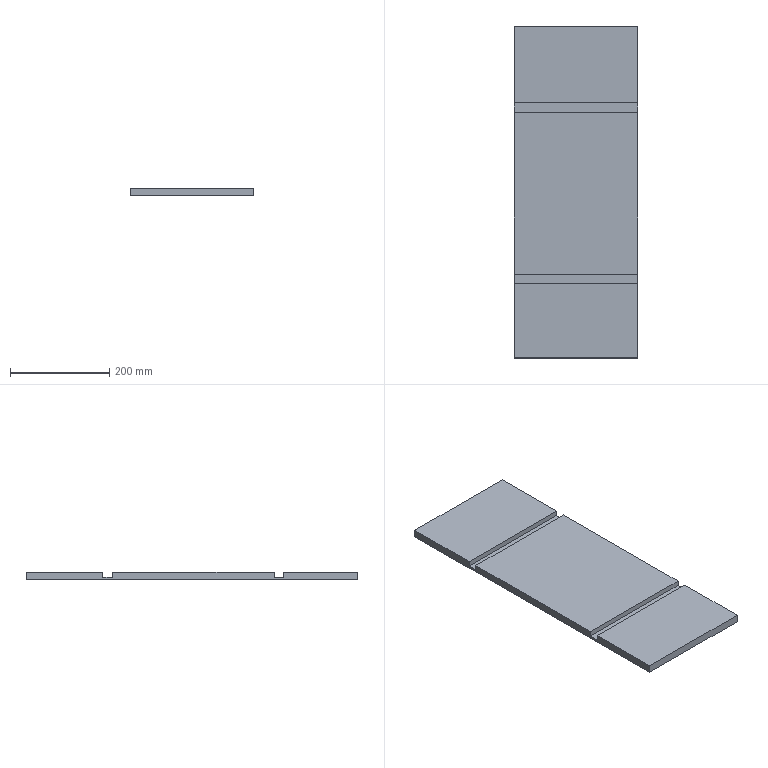Part | STEP file | Superstructure_3 | 1 solid | 14 faces | box 250 x 670 x 16 mm | volume 2577227 mm3 | plane 14
STEP:
#1=CARTESIAN_POINT('',(0.,0.,0.));
#2=DIRECTION('',(0.,0.,1.));
#3=DIRECTION('',(1.,0.,0.));
#4=AXIS2_PLACEMENT_3D('',#1,#2,#3);
#5=CARTESIAN_POINT('',(-125.,335.,0.));
#6=VERTEX_POINT('',#5);
#7=CARTESIAN_POINT('',(-125.,335.,-16.));
#8=VERTEX_POINT('',#7);
#9=CARTESIAN_POINT('',(-125.,335.,0.));
#10=DIRECTION('',(0.,0.,-1.));
#11=VECTOR('',#10,1.);
#12=LINE('',#9,#11);
#13=CARTESIAN_POINT('',(-125.,335.,0.));
#14=DIRECTION('',(1.,0.,0.));
#15=DIRECTION('',(0.,0.,-1.));
#16=AXIS2_PLACEMENT_3D('',#13,#14,#15);
#17=PLANE('',#16);
#18=CARTESIAN_POINT('',(0.,0.));
#19=DIRECTION('',(1.,0.));
#20=VECTOR('',#19,1.);
#21=LINE('',#18,#20);
#22=(GEOMETRIC_REPRESENTATION_CONTEXT(2)PARAMETRIC_REPRESENTATION_CONTEXT()REPRESENTATION_CONTEXT('',''));
#23=DEFINITIONAL_REPRESENTATION('',(#21),#22);
#24=PCURVE('',#17,#23);
#25=CARTESIAN_POINT('',(0.,335.,-8.));
#26=DIRECTION('',(0.,1.,0.));
#27=DIRECTION('',(0.,0.,1.));
#28=AXIS2_PLACEMENT_3D('',#25,#26,#27);
#29=PLANE('',#28);
#30=CARTESIAN_POINT('',(8.,-125.));
#31=DIRECTION('',(-1.,0.));
#32=VECTOR('',#31,1.);
#33=LINE('',#30,#32);
#34=(GEOMETRIC_REPRESENTATION_CONTEXT(2)PARAMETRIC_REPRESENTATION_CONTEXT()REPRESENTATION_CONTEXT('',''));
#35=DEFINITIONAL_REPRESENTATION('',(#33),#34);
#36=PCURVE('',#29,#35);
#37=SURFACE_CURVE('',#12,(#24,#36),.PCURVE_S1.);
#38=EDGE_CURVE('',#6,#8,#37,.T.);
#39=ORIENTED_EDGE('',*,*,#38,.F.);
#40=CARTESIAN_POINT('',(-125.,180.,0.));
#41=VERTEX_POINT('',#40);
#42=CARTESIAN_POINT('',(-125.,335.,0.));
#43=DIRECTION('',(0.,-1.,0.));
#44=VECTOR('',#43,1.);
#45=LINE('',#42,#44);
#46=CARTESIAN_POINT('',(0.,0.));
#47=DIRECTION('',(0.,-1.));
#48=VECTOR('',#47,1.);
#49=LINE('',#46,#48);
#50=(GEOMETRIC_REPRESENTATION_CONTEXT(2)PARAMETRIC_REPRESENTATION_CONTEXT()REPRESENTATION_CONTEXT('',''));
#51=DEFINITIONAL_REPRESENTATION('',(#49),#50);
#52=PCURVE('',#17,#51);
#53=CARTESIAN_POINT('',(125.,335.,0.));
#54=DIRECTION('',(0.,0.,-1.));
#55=DIRECTION('',(-1.,0.,0.));
#56=AXIS2_PLACEMENT_3D('',#53,#54,#55);
#57=PLANE('',#56);
#58=CARTESIAN_POINT('',(250.,0.));
#59=DIRECTION('',(0.,-1.));
#60=VECTOR('',#59,1.);
#61=LINE('',#58,#60);
#62=(GEOMETRIC_REPRESENTATION_CONTEXT(2)PARAMETRIC_REPRESENTATION_CONTEXT()REPRESENTATION_CONTEXT('',''));
#63=DEFINITIONAL_REPRESENTATION('',(#61),#62);
#64=PCURVE('',#57,#63);
#65=SURFACE_CURVE('',#45,(#52,#64),.PCURVE_S1.);
#66=EDGE_CURVE('',#6,#41,#65,.T.);
#67=ORIENTED_EDGE('',*,*,#66,.T.);
#68=CARTESIAN_POINT('',(-125.,180.,-10.65));
#69=VERTEX_POINT('',#68);
#70=CARTESIAN_POINT('',(-125.,180.,-2.663));
#71=DIRECTION('',(0.,0.,1.));
#72=VECTOR('',#71,1.);
#73=LINE('',#70,#72);
#74=CARTESIAN_POINT('',(2.663,-155.));
#75=DIRECTION('',(-1.,0.));
#76=VECTOR('',#75,1.);
#77=LINE('',#74,#76);
#78=(GEOMETRIC_REPRESENTATION_CONTEXT(2)PARAMETRIC_REPRESENTATION_CONTEXT()REPRESENTATION_CONTEXT('',''));
#79=DEFINITIONAL_REPRESENTATION('',(#77),#78);
#80=PCURVE('',#17,#79);
#81=CARTESIAN_POINT('',(0.,180.,-5.325));
#82=DIRECTION('',(0.,1.,0.));
#83=DIRECTION('',(0.,0.,1.));
#84=AXIS2_PLACEMENT_3D('',#81,#82,#83);
#85=PLANE('',#84);
#86=CARTESIAN_POINT('',(2.663,-125.));
#87=DIRECTION('',(1.,0.));
#88=VECTOR('',#87,1.);
#89=LINE('',#86,#88);
#90=(GEOMETRIC_REPRESENTATION_CONTEXT(2)PARAMETRIC_REPRESENTATION_CONTEXT()REPRESENTATION_CONTEXT('',''));
#91=DEFINITIONAL_REPRESENTATION('',(#89),#90);
#92=PCURVE('',#85,#91);
#93=SURFACE_CURVE('',#73,(#80,#92),.PCURVE_S1.);
#94=EDGE_CURVE('',#69,#41,#93,.T.);
#95=ORIENTED_EDGE('',*,*,#94,.F.);
#96=CARTESIAN_POINT('',(-125.,160.7,-10.65));
#97=VERTEX_POINT('',#96);
#98=CARTESIAN_POINT('',(-125.,252.675,-10.65));
#99=DIRECTION('',(0.,1.,0.));
#100=VECTOR('',#99,1.);
#101=LINE('',#98,#100);
#102=CARTESIAN_POINT('',(10.65,-82.325));
#103=DIRECTION('',(0.,1.));
#104=VECTOR('',#103,1.);
#105=LINE('',#102,#104);
#106=(GEOMETRIC_REPRESENTATION_CONTEXT(2)PARAMETRIC_REPRESENTATION_CONTEXT()REPRESENTATION_CONTEXT('',''));
#107=DEFINITIONAL_REPRESENTATION('',(#105),#106);
#108=PCURVE('',#17,#107);
#109=CARTESIAN_POINT('',(0.,170.35,-10.65));
#110=DIRECTION('',(0.,0.,-1.));
#111=DIRECTION('',(-1.,0.,0.));
#112=AXIS2_PLACEMENT_3D('',#109,#110,#111);
#113=PLANE('',#112);
#114=CARTESIAN_POINT('',(125.,82.325));
#115=DIRECTION('',(0.,1.));
#116=VECTOR('',#115,1.);
#117=LINE('',#114,#116);
#118=(GEOMETRIC_REPRESENTATION_CONTEXT(2)PARAMETRIC_REPRESENTATION_CONTEXT()REPRESENTATION_CONTEXT('',''));
#119=DEFINITIONAL_REPRESENTATION('',(#117),#118);
#120=PCURVE('',#113,#119);
#121=SURFACE_CURVE('',#101,(#108,#120),.PCURVE_S1.);
#122=EDGE_CURVE('',#97,#69,#121,.T.);
#123=ORIENTED_EDGE('',*,*,#122,.F.);
#124=CARTESIAN_POINT('',(-125.,160.7,0.));
#125=VERTEX_POINT('',#124);
#126=CARTESIAN_POINT('',(-125.,160.7,-2.663));
#127=DIRECTION('',(0.,0.,-1.));
#128=VECTOR('',#127,1.);
#129=LINE('',#126,#128);
#130=CARTESIAN_POINT('',(2.663,-174.3));
#131=DIRECTION('',(1.,0.));
#132=VECTOR('',#131,1.);
#133=LINE('',#130,#132);
#134=(GEOMETRIC_REPRESENTATION_CONTEXT(2)PARAMETRIC_REPRESENTATION_CONTEXT()REPRESENTATION_CONTEXT('',''));
#135=DEFINITIONAL_REPRESENTATION('',(#133),#134);
#136=PCURVE('',#17,#135);
#137=CARTESIAN_POINT('',(0.,160.7,-5.325));
#138=DIRECTION('',(0.,-1.,0.));
#139=DIRECTION('',(0.,0.,-1.));
#140=AXIS2_PLACEMENT_3D('',#137,#138,#139);
#141=PLANE('',#140);
#142=CARTESIAN_POINT('',(-2.663,-125.));
#143=DIRECTION('',(1.,0.));
#144=VECTOR('',#143,1.);
#145=LINE('',#142,#144);
#146=(GEOMETRIC_REPRESENTATION_CONTEXT(2)PARAMETRIC_REPRESENTATION_CONTEXT()REPRESENTATION_CONTEXT('',''));
#147=DEFINITIONAL_REPRESENTATION('',(#145),#146);
#148=PCURVE('',#141,#147);
#149=SURFACE_CURVE('',#129,(#136,#148),.PCURVE_S1.);
#150=EDGE_CURVE('',#125,#97,#149,.T.);
#151=ORIENTED_EDGE('',*,*,#150,.F.);
#152=CARTESIAN_POINT('',(-125.,-166.2,0.));
#153=VERTEX_POINT('',#152);
#154=CARTESIAN_POINT('',(-125.,335.,0.));
#155=DIRECTION('',(0.,-1.,0.));
#156=VECTOR('',#155,1.);
#157=LINE('',#154,#156);
#158=CARTESIAN_POINT('',(0.,0.));
#159=DIRECTION('',(0.,-1.));
#160=VECTOR('',#159,1.);
#161=LINE('',#158,#160);
#162=(GEOMETRIC_REPRESENTATION_CONTEXT(2)PARAMETRIC_REPRESENTATION_CONTEXT()REPRESENTATION_CONTEXT('',''));
#163=DEFINITIONAL_REPRESENTATION('',(#161),#162);
#164=PCURVE('',#17,#163);
#165=CARTESIAN_POINT('',(125.,335.,0.));
#166=DIRECTION('',(0.,0.,-1.));
#167=DIRECTION('',(-1.,0.,0.));
#168=AXIS2_PLACEMENT_3D('',#165,#166,#167);
#169=PLANE('',#168);
#170=CARTESIAN_POINT('',(250.,0.));
#171=DIRECTION('',(0.,-1.));
#172=VECTOR('',#171,1.);
#173=LINE('',#170,#172);
#174=(GEOMETRIC_REPRESENTATION_CONTEXT(2)PARAMETRIC_REPRESENTATION_CONTEXT()REPRESENTATION_CONTEXT('',''));
#175=DEFINITIONAL_REPRESENTATION('',(#173),#174);
#176=PCURVE('',#169,#175);
#177=SURFACE_CURVE('',#157,(#164,#176),.PCURVE_S1.);
#178=EDGE_CURVE('',#125,#153,#177,.T.);
#179=ORIENTED_EDGE('',*,*,#178,.T.);
#180=CARTESIAN_POINT('',(-125.,-166.2,-10.65));
#181=VERTEX_POINT('',#180);
#182=CARTESIAN_POINT('',(-125.,-166.2,-2.663));
#183=DIRECTION('',(0.,0.,1.));
#184=VECTOR('',#183,1.);
#185=LINE('',#182,#184);
#186=CARTESIAN_POINT('',(2.663,-501.2));
#187=DIRECTION('',(-1.,0.));
#188=VECTOR('',#187,1.);
#189=LINE('',#186,#188);
#190=(GEOMETRIC_REPRESENTATION_CONTEXT(2)PARAMETRIC_REPRESENTATION_CONTEXT()REPRESENTATION_CONTEXT('',''));
#191=DEFINITIONAL_REPRESENTATION('',(#189),#190);
#192=PCURVE('',#17,#191);
#193=CARTESIAN_POINT('',(0.,-166.2,-5.325));
#194=DIRECTION('',(0.,1.,0.));
#195=DIRECTION('',(0.,0.,1.));
#196=AXIS2_PLACEMENT_3D('',#193,#194,#195);
#197=PLANE('',#196);
#198=CARTESIAN_POINT('',(2.663,-125.));
#199=DIRECTION('',(1.,0.));
#200=VECTOR('',#199,1.);
#201=LINE('',#198,#200);
#202=(GEOMETRIC_REPRESENTATION_CONTEXT(2)PARAMETRIC_REPRESENTATION_CONTEXT()REPRESENTATION_CONTEXT('',''));
#203=DEFINITIONAL_REPRESENTATION('',(#201),#202);
#204=PCURVE('',#197,#203);
#205=SURFACE_CURVE('',#185,(#192,#204),.PCURVE_S1.);
#206=EDGE_CURVE('',#181,#153,#205,.T.);
#207=ORIENTED_EDGE('',*,*,#206,.F.);
#208=CARTESIAN_POINT('',(-125.,-185.5,-10.65));
#209=VERTEX_POINT('',#208);
#210=CARTESIAN_POINT('',(-125.,79.575,-10.65));
#211=DIRECTION('',(0.,1.,0.));
#212=VECTOR('',#211,1.);
#213=LINE('',#210,#212);
#214=CARTESIAN_POINT('',(10.65,-255.425));
#215=DIRECTION('',(0.,1.));
#216=VECTOR('',#215,1.);
#217=LINE('',#214,#216);
#218=(GEOMETRIC_REPRESENTATION_CONTEXT(2)PARAMETRIC_REPRESENTATION_CONTEXT()REPRESENTATION_CONTEXT('',''));
#219=DEFINITIONAL_REPRESENTATION('',(#217),#218);
#220=PCURVE('',#17,#219);
#221=CARTESIAN_POINT('',(0.,-175.85,-10.65));
#222=DIRECTION('',(0.,0.,-1.));
#223=DIRECTION('',(-1.,0.,0.));
#224=AXIS2_PLACEMENT_3D('',#221,#222,#223);
#225=PLANE('',#224);
#226=CARTESIAN_POINT('',(125.,255.425));
#227=DIRECTION('',(0.,1.));
#228=VECTOR('',#227,1.);
#229=LINE('',#226,#228);
#230=(GEOMETRIC_REPRESENTATION_CONTEXT(2)PARAMETRIC_REPRESENTATION_CONTEXT()REPRESENTATION_CONTEXT('',''));
#231=DEFINITIONAL_REPRESENTATION('',(#229),#230);
#232=PCURVE('',#225,#231);
#233=SURFACE_CURVE('',#213,(#220,#232),.PCURVE_S1.);
#234=EDGE_CURVE('',#209,#181,#233,.T.);
#235=ORIENTED_EDGE('',*,*,#234,.F.);
#236=CARTESIAN_POINT('',(-125.,-185.5,0.));
#237=VERTEX_POINT('',#236);
#238=CARTESIAN_POINT('',(-125.,-185.5,-2.663));
#239=DIRECTION('',(0.,0.,-1.));
#240=VECTOR('',#239,1.);
#241=LINE('',#238,#240);
#242=CARTESIAN_POINT('',(2.663,-520.5));
#243=DIRECTION('',(1.,0.));
#244=VECTOR('',#243,1.);
#245=LINE('',#242,#244);
#246=(GEOMETRIC_REPRESENTATION_CONTEXT(2)PARAMETRIC_REPRESENTATION_CONTEXT()REPRESENTATION_CONTEXT('',''));
#247=DEFINITIONAL_REPRESENTATION('',(#245),#246);
#248=PCURVE('',#17,#247);
#249=CARTESIAN_POINT('',(0.,-185.5,-5.325));
#250=DIRECTION('',(0.,-1.,0.));
#251=DIRECTION('',(0.,0.,-1.));
#252=AXIS2_PLACEMENT_3D('',#249,#250,#251);
#253=PLANE('',#252);
#254=CARTESIAN_POINT('',(-2.663,-125.));
#255=DIRECTION('',(1.,0.));
#256=VECTOR('',#255,1.);
#257=LINE('',#254,#256);
#258=(GEOMETRIC_REPRESENTATION_CONTEXT(2)PARAMETRIC_REPRESENTATION_CONTEXT()REPRESENTATION_CONTEXT('',''));
#259=DEFINITIONAL_REPRESENTATION('',(#257),#258);
#260=PCURVE('',#253,#259);
#261=SURFACE_CURVE('',#241,(#248,#260),.PCURVE_S1.);
#262=EDGE_CURVE('',#237,#209,#261,.T.);
#263=ORIENTED_EDGE('',*,*,#262,.F.);
#264=CARTESIAN_POINT('',(-125.,-335.,0.));
#265=VERTEX_POINT('',#264);
#266=CARTESIAN_POINT('',(-125.,335.,0.));
#267=DIRECTION('',(0.,-1.,0.));
#268=VECTOR('',#267,1.);
#269=LINE('',#266,#268);
#270=CARTESIAN_POINT('',(0.,0.));
#271=DIRECTION('',(0.,-1.));
#272=VECTOR('',#271,1.);
#273=LINE('',#270,#272);
#274=(GEOMETRIC_REPRESENTATION_CONTEXT(2)PARAMETRIC_REPRESENTATION_CONTEXT()REPRESENTATION_CONTEXT('',''));
#275=DEFINITIONAL_REPRESENTATION('',(#273),#274);
#276=PCURVE('',#17,#275);
#277=CARTESIAN_POINT('',(125.,335.,0.));
#278=DIRECTION('',(0.,0.,-1.));
#279=DIRECTION('',(-1.,0.,0.));
#280=AXIS2_PLACEMENT_3D('',#277,#278,#279);
#281=PLANE('',#280);
#282=CARTESIAN_POINT('',(250.,0.));
#283=DIRECTION('',(0.,-1.));
#284=VECTOR('',#283,1.);
#285=LINE('',#282,#284);
#286=(GEOMETRIC_REPRESENTATION_CONTEXT(2)PARAMETRIC_REPRESENTATION_CONTEXT()REPRESENTATION_CONTEXT('',''));
#287=DEFINITIONAL_REPRESENTATION('',(#285),#286);
#288=PCURVE('',#281,#287);
#289=SURFACE_CURVE('',#269,(#276,#288),.PCURVE_S1.);
#290=EDGE_CURVE('',#237,#265,#289,.T.);
#291=ORIENTED_EDGE('',*,*,#290,.T.);
#292=CARTESIAN_POINT('',(-125.,-335.,-16.));
#293=VERTEX_POINT('',#292);
#294=CARTESIAN_POINT('',(-125.,-335.,0.));
#295=DIRECTION('',(0.,0.,-1.));
#296=VECTOR('',#295,1.);
#297=LINE('',#294,#296);
#298=CARTESIAN_POINT('',(0.,-670.));
#299=DIRECTION('',(1.,0.));
#300=VECTOR('',#299,1.);
#301=LINE('',#298,#300);
#302=(GEOMETRIC_REPRESENTATION_CONTEXT(2)PARAMETRIC_REPRESENTATION_CONTEXT()REPRESENTATION_CONTEXT('',''));
#303=DEFINITIONAL_REPRESENTATION('',(#301),#302);
#304=PCURVE('',#17,#303);
#305=CARTESIAN_POINT('',(0.,-335.,-8.));
#306=DIRECTION('',(0.,1.,0.));
#307=DIRECTION('',(0.,0.,1.));
#308=AXIS2_PLACEMENT_3D('',#305,#306,#307);
#309=PLANE('',#308);
#310=CARTESIAN_POINT('',(8.,-125.));
#311=DIRECTION('',(-1.,0.));
#312=VECTOR('',#311,1.);
#313=LINE('',#310,#312);
#314=(GEOMETRIC_REPRESENTATION_CONTEXT(2)PARAMETRIC_REPRESENTATION_CONTEXT()REPRESENTATION_CONTEXT('',''));
#315=DEFINITIONAL_REPRESENTATION('',(#313),#314);
#316=PCURVE('',#309,#315);
#317=SURFACE_CURVE('',#297,(#304,#316),.PCURVE_S1.);
#318=EDGE_CURVE('',#265,#293,#317,.T.);
#319=ORIENTED_EDGE('',*,*,#318,.T.);
#320=CARTESIAN_POINT('',(-125.,335.,-16.));
#321=DIRECTION('',(0.,-1.,0.));
#322=VECTOR('',#321,1.);
#323=LINE('',#320,#322);
#324=CARTESIAN_POINT('',(16.,0.));
#325=DIRECTION('',(0.,-1.));
#326=VECTOR('',#325,1.);
#327=LINE('',#324,#326);
#328=(GEOMETRIC_REPRESENTATION_CONTEXT(2)PARAMETRIC_REPRESENTATION_CONTEXT()REPRESENTATION_CONTEXT('',''));
#329=DEFINITIONAL_REPRESENTATION('',(#327),#328);
#330=PCURVE('',#17,#329);
#331=CARTESIAN_POINT('',(-125.,335.,-16.));
#332=DIRECTION('',(0.,0.,1.));
#333=DIRECTION('',(1.,0.,0.));
#334=AXIS2_PLACEMENT_3D('',#331,#332,#333);
#335=PLANE('',#334);
#336=CARTESIAN_POINT('',(0.,0.));
#337=DIRECTION('',(0.,-1.));
#338=VECTOR('',#337,1.);
#339=LINE('',#336,#338);
#340=(GEOMETRIC_REPRESENTATION_CONTEXT(2)PARAMETRIC_REPRESENTATION_CONTEXT()REPRESENTATION_CONTEXT('',''));
#341=DEFINITIONAL_REPRESENTATION('',(#339),#340);
#342=PCURVE('',#335,#341);
#343=SURFACE_CURVE('',#323,(#330,#342),.PCURVE_S1.);
#344=EDGE_CURVE('',#8,#293,#343,.T.);
#345=ORIENTED_EDGE('',*,*,#344,.F.);
#346=EDGE_LOOP('',(#39,#67,#95,#123,#151,#179,#207,#235,#263,#291,#319,#345));
#347=FACE_BOUND('',#346,.F.);
#348=ADVANCED_FACE('',(#347),#17,.F.);
#349=ORIENTED_EDGE('',*,*,#38,.T.);
#350=CARTESIAN_POINT('',(125.,335.,-16.));
#351=VERTEX_POINT('',#350);
#352=CARTESIAN_POINT('',(-125.,335.,-16.));
#353=DIRECTION('',(1.,0.,0.));
#354=VECTOR('',#353,1.);
#355=LINE('',#352,#354);
#356=CARTESIAN_POINT('',(-8.,-125.));
#357=DIRECTION('',(0.,1.));
#358=VECTOR('',#357,1.);
#359=LINE('',#356,#358);
#360=(GEOMETRIC_REPRESENTATION_CONTEXT(2)PARAMETRIC_REPRESENTATION_CONTEXT()REPRESENTATION_CONTEXT('',''));
#361=DEFINITIONAL_REPRESENTATION('',(#359),#360);
#362=PCURVE('',#29,#361);
#363=CARTESIAN_POINT('',(0.,0.));
#364=DIRECTION('',(1.,0.));
#365=VECTOR('',#364,1.);
#366=LINE('',#363,#365);
#367=(GEOMETRIC_REPRESENTATION_CONTEXT(2)PARAMETRIC_REPRESENTATION_CONTEXT()REPRESENTATION_CONTEXT('',''));
#368=DEFINITIONAL_REPRESENTATION('',(#366),#367);
#369=PCURVE('',#335,#368);
#370=SURFACE_CURVE('',#355,(#362,#369),.PCURVE_S1.);
#371=EDGE_CURVE('',#8,#351,#370,.T.);
#372=ORIENTED_EDGE('',*,*,#371,.T.);
#373=CARTESIAN_POINT('',(125.,335.,0.));
#374=VERTEX_POINT('',#373);
#375=CARTESIAN_POINT('',(125.,335.,-16.));
#376=DIRECTION('',(0.,0.,1.));
#377=VECTOR('',#376,1.);
#378=LINE('',#375,#377);
#379=CARTESIAN_POINT('',(-8.,125.));
#380=DIRECTION('',(1.,0.));
#381=VECTOR('',#380,1.);
#382=LINE('',#379,#381);
#383=(GEOMETRIC_REPRESENTATION_CONTEXT(2)PARAMETRIC_REPRESENTATION_CONTEXT()REPRESENTATION_CONTEXT('',''));
#384=DEFINITIONAL_REPRESENTATION('',(#382),#383);
#385=PCURVE('',#29,#384);
#386=CARTESIAN_POINT('',(125.,335.,-16.));
#387=DIRECTION('',(-1.,0.,0.));
#388=DIRECTION('',(0.,0.,1.));
#389=AXIS2_PLACEMENT_3D('',#386,#387,#388);
#390=PLANE('',#389);
#391=CARTESIAN_POINT('',(0.,0.));
#392=DIRECTION('',(1.,0.));
#393=VECTOR('',#392,1.);
#394=LINE('',#391,#393);
#395=(GEOMETRIC_REPRESENTATION_CONTEXT(2)PARAMETRIC_REPRESENTATION_CONTEXT()REPRESENTATION_CONTEXT('',''));
#396=DEFINITIONAL_REPRESENTATION('',(#394),#395);
#397=PCURVE('',#390,#396);
#398=SURFACE_CURVE('',#378,(#385,#397),.PCURVE_S1.);
#399=EDGE_CURVE('',#351,#374,#398,.T.);
#400=ORIENTED_EDGE('',*,*,#399,.T.);
#401=CARTESIAN_POINT('',(125.,335.,0.));
#402=DIRECTION('',(-1.,0.,0.));
#403=VECTOR('',#402,1.);
#404=LINE('',#401,#403);
#405=CARTESIAN_POINT('',(8.,125.));
#406=DIRECTION('',(0.,-1.));
#407=VECTOR('',#406,1.);
#408=LINE('',#405,#407);
#409=(GEOMETRIC_REPRESENTATION_CONTEXT(2)PARAMETRIC_REPRESENTATION_CONTEXT()REPRESENTATION_CONTEXT('',''));
#410=DEFINITIONAL_REPRESENTATION('',(#408),#409);
#411=PCURVE('',#29,#410);
#412=CARTESIAN_POINT('',(0.,0.));
#413=DIRECTION('',(1.,0.));
#414=VECTOR('',#413,1.);
#415=LINE('',#412,#414);
#416=(GEOMETRIC_REPRESENTATION_CONTEXT(2)PARAMETRIC_REPRESENTATION_CONTEXT()REPRESENTATION_CONTEXT('',''));
#417=DEFINITIONAL_REPRESENTATION('',(#415),#416);
#418=PCURVE('',#57,#417);
#419=SURFACE_CURVE('',#404,(#411,#418),.PCURVE_S1.);
#420=EDGE_CURVE('',#374,#6,#419,.T.);
#421=ORIENTED_EDGE('',*,*,#420,.T.);
#422=EDGE_LOOP('',(#349,#372,#400,#421));
#423=FACE_BOUND('',#422,.F.);
#424=ADVANCED_FACE('',(#423),#29,.T.);
#425=ORIENTED_EDGE('',*,*,#344,.T.);
#426=CARTESIAN_POINT('',(125.,-335.,-16.));
#427=VERTEX_POINT('',#426);
#428=CARTESIAN_POINT('',(-125.,-335.,-16.));
#429=DIRECTION('',(1.,0.,0.));
#430=VECTOR('',#429,1.);
#431=LINE('',#428,#430);
#432=CARTESIAN_POINT('',(0.,-670.));
#433=DIRECTION('',(1.,0.));
#434=VECTOR('',#433,1.);
#435=LINE('',#432,#434);
#436=(GEOMETRIC_REPRESENTATION_CONTEXT(2)PARAMETRIC_REPRESENTATION_CONTEXT()REPRESENTATION_CONTEXT('',''));
#437=DEFINITIONAL_REPRESENTATION('',(#435),#436);
#438=PCURVE('',#335,#437);
#439=CARTESIAN_POINT('',(-8.,-125.));
#440=DIRECTION('',(0.,1.));
#441=VECTOR('',#440,1.);
#442=LINE('',#439,#441);
#443=(GEOMETRIC_REPRESENTATION_CONTEXT(2)PARAMETRIC_REPRESENTATION_CONTEXT()REPRESENTATION_CONTEXT('',''));
#444=DEFINITIONAL_REPRESENTATION('',(#442),#443);
#445=PCURVE('',#309,#444);
#446=SURFACE_CURVE('',#431,(#438,#445),.PCURVE_S1.);
#447=EDGE_CURVE('',#293,#427,#446,.T.);
#448=ORIENTED_EDGE('',*,*,#447,.T.);
#449=CARTESIAN_POINT('',(125.,335.,-16.));
#450=DIRECTION('',(0.,-1.,0.));
#451=VECTOR('',#450,1.);
#452=LINE('',#449,#451);
#453=CARTESIAN_POINT('',(250.,0.));
#454=DIRECTION('',(0.,-1.));
#455=VECTOR('',#454,1.);
#456=LINE('',#453,#455);
#457=(GEOMETRIC_REPRESENTATION_CONTEXT(2)PARAMETRIC_REPRESENTATION_CONTEXT()REPRESENTATION_CONTEXT('',''));
#458=DEFINITIONAL_REPRESENTATION('',(#456),#457);
#459=PCURVE('',#335,#458);
#460=CARTESIAN_POINT('',(0.,0.));
#461=DIRECTION('',(0.,-1.));
#462=VECTOR('',#461,1.);
#463=LINE('',#460,#462);
#464=(GEOMETRIC_REPRESENTATION_CONTEXT(2)PARAMETRIC_REPRESENTATION_CONTEXT()REPRESENTATION_CONTEXT('',''));
#465=DEFINITIONAL_REPRESENTATION('',(#463),#464);
#466=PCURVE('',#390,#465);
#467=SURFACE_CURVE('',#452,(#459,#466),.PCURVE_S1.);
#468=EDGE_CURVE('',#351,#427,#467,.T.);
#469=ORIENTED_EDGE('',*,*,#468,.F.);
#470=ORIENTED_EDGE('',*,*,#371,.F.);
#471=EDGE_LOOP('',(#425,#448,#469,#470));
#472=FACE_BOUND('',#471,.F.);
#473=ADVANCED_FACE('',(#472),#335,.F.);
#474=ORIENTED_EDGE('',*,*,#318,.T.);
#475=ORIENTED_EDGE('',*,*,#447,.T.);
#476=CARTESIAN_POINT('',(125.,-335.,0.));
#477=VERTEX_POINT('',#476);
#478=CARTESIAN_POINT('',(125.,-335.,-16.));
#479=DIRECTION('',(0.,0.,1.));
#480=VECTOR('',#479,1.);
#481=LINE('',#478,#480);
#482=CARTESIAN_POINT('',(-8.,125.));
#483=DIRECTION('',(1.,0.));
#484=VECTOR('',#483,1.);
#485=LINE('',#482,#484);
#486=(GEOMETRIC_REPRESENTATION_CONTEXT(2)PARAMETRIC_REPRESENTATION_CONTEXT()REPRESENTATION_CONTEXT('',''));
#487=DEFINITIONAL_REPRESENTATION('',(#485),#486);
#488=PCURVE('',#309,#487);
#489=CARTESIAN_POINT('',(0.,-670.));
#490=DIRECTION('',(1.,0.));
#491=VECTOR('',#490,1.);
#492=LINE('',#489,#491);
#493=(GEOMETRIC_REPRESENTATION_CONTEXT(2)PARAMETRIC_REPRESENTATION_CONTEXT()REPRESENTATION_CONTEXT('',''));
#494=DEFINITIONAL_REPRESENTATION('',(#492),#493);
#495=PCURVE('',#390,#494);
#496=SURFACE_CURVE('',#481,(#488,#495),.PCURVE_S1.);
#497=EDGE_CURVE('',#427,#477,#496,.T.);
#498=ORIENTED_EDGE('',*,*,#497,.T.);
#499=CARTESIAN_POINT('',(125.,-335.,0.));
#500=DIRECTION('',(-1.,0.,0.));
#501=VECTOR('',#500,1.);
#502=LINE('',#499,#501);
#503=CARTESIAN_POINT('',(8.,125.));
#504=DIRECTION('',(0.,-1.));
#505=VECTOR('',#504,1.);
#506=LINE('',#503,#505);
#507=(GEOMETRIC_REPRESENTATION_CONTEXT(2)PARAMETRIC_REPRESENTATION_CONTEXT()REPRESENTATION_CONTEXT('',''));
#508=DEFINITIONAL_REPRESENTATION('',(#506),#507);
#509=PCURVE('',#309,#508);
#510=CARTESIAN_POINT('',(0.,-670.));
#511=DIRECTION('',(1.,0.));
#512=VECTOR('',#511,1.);
#513=LINE('',#510,#512);
#514=(GEOMETRIC_REPRESENTATION_CONTEXT(2)PARAMETRIC_REPRESENTATION_CONTEXT()REPRESENTATION_CONTEXT('',''));
#515=DEFINITIONAL_REPRESENTATION('',(#513),#514);
#516=PCURVE('',#281,#515);
#517=SURFACE_CURVE('',#502,(#509,#516),.PCURVE_S1.);
#518=EDGE_CURVE('',#477,#265,#517,.T.);
#519=ORIENTED_EDGE('',*,*,#518,.T.);
#520=EDGE_LOOP('',(#474,#475,#498,#519));
#521=FACE_BOUND('',#520,.T.);
#522=ADVANCED_FACE('',(#521),#309,.F.);
#523=CARTESIAN_POINT('',(125.,-185.5,0.));
#524=VERTEX_POINT('',#523);
#525=CARTESIAN_POINT('',(0.,-185.5,0.));
#526=DIRECTION('',(1.,0.,0.));
#527=VECTOR('',#526,1.);
#528=LINE('',#525,#527);
#529=CARTESIAN_POINT('',(125.,-520.5));
#530=DIRECTION('',(-1.,0.));
#531=VECTOR('',#530,1.);
#532=LINE('',#529,#531);
#533=(GEOMETRIC_REPRESENTATION_CONTEXT(2)PARAMETRIC_REPRESENTATION_CONTEXT()REPRESENTATION_CONTEXT('',''));
#534=DEFINITIONAL_REPRESENTATION('',(#532),#533);
#535=PCURVE('',#281,#534);
#536=CARTESIAN_POINT('',(-5.325,0.));
#537=DIRECTION('',(0.,1.));
#538=VECTOR('',#537,1.);
#539=LINE('',#536,#538);
#540=(GEOMETRIC_REPRESENTATION_CONTEXT(2)PARAMETRIC_REPRESENTATION_CONTEXT()REPRESENTATION_CONTEXT('',''));
#541=DEFINITIONAL_REPRESENTATION('',(#539),#540);
#542=PCURVE('',#253,#541);
#543=SURFACE_CURVE('',#528,(#535,#542),.PCURVE_S1.);
#544=EDGE_CURVE('',#237,#524,#543,.T.);
#545=ORIENTED_EDGE('',*,*,#544,.T.);
#546=CARTESIAN_POINT('',(125.,335.,0.));
#547=DIRECTION('',(0.,-1.,0.));
#548=VECTOR('',#547,1.);
#549=LINE('',#546,#548);
#550=CARTESIAN_POINT('',(0.,0.));
#551=DIRECTION('',(0.,-1.));
#552=VECTOR('',#551,1.);
#553=LINE('',#550,#552);
#554=(GEOMETRIC_REPRESENTATION_CONTEXT(2)PARAMETRIC_REPRESENTATION_CONTEXT()REPRESENTATION_CONTEXT('',''));
#555=DEFINITIONAL_REPRESENTATION('',(#553),#554);
#556=PCURVE('',#281,#555);
#557=CARTESIAN_POINT('',(16.,0.));
#558=DIRECTION('',(0.,-1.));
#559=VECTOR('',#558,1.);
#560=LINE('',#557,#559);
#561=(GEOMETRIC_REPRESENTATION_CONTEXT(2)PARAMETRIC_REPRESENTATION_CONTEXT()REPRESENTATION_CONTEXT('',''));
#562=DEFINITIONAL_REPRESENTATION('',(#560),#561);
#563=PCURVE('',#390,#562);
#564=SURFACE_CURVE('',#549,(#556,#563),.PCURVE_S1.);
#565=EDGE_CURVE('',#524,#477,#564,.T.);
#566=ORIENTED_EDGE('',*,*,#565,.T.);
#567=ORIENTED_EDGE('',*,*,#518,.T.);
#568=ORIENTED_EDGE('',*,*,#290,.F.);
#569=EDGE_LOOP('',(#545,#566,#567,#568));
#570=FACE_BOUND('',#569,.F.);
#571=ADVANCED_FACE('',(#570),#281,.F.);
#572=ORIENTED_EDGE('',*,*,#544,.F.);
#573=ORIENTED_EDGE('',*,*,#262,.T.);
#574=CARTESIAN_POINT('',(125.,-185.5,-10.65));
#575=VERTEX_POINT('',#574);
#576=CARTESIAN_POINT('',(0.,-185.5,-10.65));
#577=DIRECTION('',(-1.,0.,0.));
#578=VECTOR('',#577,1.);
#579=LINE('',#576,#578);
#580=CARTESIAN_POINT('',(5.325,0.));
#581=DIRECTION('',(0.,-1.));
#582=VECTOR('',#581,1.);
#583=LINE('',#580,#582);
#584=(GEOMETRIC_REPRESENTATION_CONTEXT(2)PARAMETRIC_REPRESENTATION_CONTEXT()REPRESENTATION_CONTEXT('',''));
#585=DEFINITIONAL_REPRESENTATION('',(#583),#584);
#586=PCURVE('',#253,#585);
#587=CARTESIAN_POINT('',(0.,-9.65));
#588=DIRECTION('',(1.,0.));
#589=VECTOR('',#588,1.);
#590=LINE('',#587,#589);
#591=(GEOMETRIC_REPRESENTATION_CONTEXT(2)PARAMETRIC_REPRESENTATION_CONTEXT()REPRESENTATION_CONTEXT('',''));
#592=DEFINITIONAL_REPRESENTATION('',(#590),#591);
#593=PCURVE('',#225,#592);
#594=SURFACE_CURVE('',#579,(#586,#593),.PCURVE_S1.);
#595=EDGE_CURVE('',#575,#209,#594,.T.);
#596=ORIENTED_EDGE('',*,*,#595,.F.);
#597=CARTESIAN_POINT('',(125.,-185.5,-10.662));
#598=DIRECTION('',(0.,0.,1.));
#599=VECTOR('',#598,1.);
#600=LINE('',#597,#599);
#601=CARTESIAN_POINT('',(5.338,125.));
#602=DIRECTION('',(-1.,0.));
#603=VECTOR('',#602,1.);
#604=LINE('',#601,#603);
#605=(GEOMETRIC_REPRESENTATION_CONTEXT(2)PARAMETRIC_REPRESENTATION_CONTEXT()REPRESENTATION_CONTEXT('',''));
#606=DEFINITIONAL_REPRESENTATION('',(#604),#605);
#607=PCURVE('',#253,#606);
#608=CARTESIAN_POINT('',(5.338,-520.5));
#609=DIRECTION('',(1.,0.));
#610=VECTOR('',#609,1.);
#611=LINE('',#608,#610);
#612=(GEOMETRIC_REPRESENTATION_CONTEXT(2)PARAMETRIC_REPRESENTATION_CONTEXT()REPRESENTATION_CONTEXT('',''));
#613=DEFINITIONAL_REPRESENTATION('',(#611),#612);
#614=PCURVE('',#390,#613);
#615=SURFACE_CURVE('',#600,(#607,#614),.PCURVE_S1.);
#616=EDGE_CURVE('',#575,#524,#615,.T.);
#617=ORIENTED_EDGE('',*,*,#616,.T.);
#618=EDGE_LOOP('',(#572,#573,#596,#617));
#619=FACE_BOUND('',#618,.F.);
#620=ADVANCED_FACE('',(#619),#253,.F.);
#621=CARTESIAN_POINT('',(125.,-166.2,-10.65));
#622=VERTEX_POINT('',#621);
#623=CARTESIAN_POINT('',(125.,79.575,-10.65));
#624=DIRECTION('',(0.,-1.,0.));
#625=VECTOR('',#624,1.);
#626=LINE('',#623,#625);
#627=CARTESIAN_POINT('',(-125.,255.425));
#628=DIRECTION('',(0.,-1.));
#629=VECTOR('',#628,1.);
#630=LINE('',#627,#629);
#631=(GEOMETRIC_REPRESENTATION_CONTEXT(2)PARAMETRIC_REPRESENTATION_CONTEXT()REPRESENTATION_CONTEXT('',''));
#632=DEFINITIONAL_REPRESENTATION('',(#630),#631);
#633=PCURVE('',#225,#632);
#634=CARTESIAN_POINT('',(5.35,-255.425));
#635=DIRECTION('',(0.,-1.));
#636=VECTOR('',#635,1.);
#637=LINE('',#634,#636);
#638=(GEOMETRIC_REPRESENTATION_CONTEXT(2)PARAMETRIC_REPRESENTATION_CONTEXT()REPRESENTATION_CONTEXT('',''));
#639=DEFINITIONAL_REPRESENTATION('',(#637),#638);
#640=PCURVE('',#390,#639);
#641=SURFACE_CURVE('',#626,(#633,#640),.PCURVE_S1.);
#642=EDGE_CURVE('',#622,#575,#641,.T.);
#643=ORIENTED_EDGE('',*,*,#642,.T.);
#644=ORIENTED_EDGE('',*,*,#595,.T.);
#645=ORIENTED_EDGE('',*,*,#234,.T.);
#646=CARTESIAN_POINT('',(0.,-166.2,-10.65));
#647=DIRECTION('',(-1.,0.,0.));
#648=VECTOR('',#647,1.);
#649=LINE('',#646,#648);
#650=CARTESIAN_POINT('',(0.,9.65));
#651=DIRECTION('',(1.,0.));
#652=VECTOR('',#651,1.);
#653=LINE('',#650,#652);
#654=(GEOMETRIC_REPRESENTATION_CONTEXT(2)PARAMETRIC_REPRESENTATION_CONTEXT()REPRESENTATION_CONTEXT('',''));
#655=DEFINITIONAL_REPRESENTATION('',(#653),#654);
#656=PCURVE('',#225,#655);
#657=CARTESIAN_POINT('',(-5.325,0.));
#658=DIRECTION('',(0.,-1.));
#659=VECTOR('',#658,1.);
#660=LINE('',#657,#659);
#661=(GEOMETRIC_REPRESENTATION_CONTEXT(2)PARAMETRIC_REPRESENTATION_CONTEXT()REPRESENTATION_CONTEXT('',''));
#662=DEFINITIONAL_REPRESENTATION('',(#660),#661);
#663=PCURVE('',#197,#662);
#664=SURFACE_CURVE('',#649,(#656,#663),.PCURVE_S1.);
#665=EDGE_CURVE('',#622,#181,#664,.T.);
#666=ORIENTED_EDGE('',*,*,#665,.F.);
#667=EDGE_LOOP('',(#643,#644,#645,#666));
#668=FACE_BOUND('',#667,.F.);
#669=ADVANCED_FACE('',(#668),#225,.F.);
#670=CARTESIAN_POINT('',(125.,-166.2,0.));
#671=VERTEX_POINT('',#670);
#672=CARTESIAN_POINT('',(125.,-166.2,-10.662));
#673=DIRECTION('',(0.,0.,-1.));
#674=VECTOR('',#673,1.);
#675=LINE('',#672,#674);
#676=CARTESIAN_POINT('',(-5.338,125.));
#677=DIRECTION('',(-1.,0.));
#678=VECTOR('',#677,1.);
#679=LINE('',#676,#678);
#680=(GEOMETRIC_REPRESENTATION_CONTEXT(2)PARAMETRIC_REPRESENTATION_CONTEXT()REPRESENTATION_CONTEXT('',''));
#681=DEFINITIONAL_REPRESENTATION('',(#679),#680);
#682=PCURVE('',#197,#681);
#683=CARTESIAN_POINT('',(5.338,-501.2));
#684=DIRECTION('',(-1.,0.));
#685=VECTOR('',#684,1.);
#686=LINE('',#683,#685);
#687=(GEOMETRIC_REPRESENTATION_CONTEXT(2)PARAMETRIC_REPRESENTATION_CONTEXT()REPRESENTATION_CONTEXT('',''));
#688=DEFINITIONAL_REPRESENTATION('',(#686),#687);
#689=PCURVE('',#390,#688);
#690=SURFACE_CURVE('',#675,(#682,#689),.PCURVE_S1.);
#691=EDGE_CURVE('',#671,#622,#690,.T.);
#692=ORIENTED_EDGE('',*,*,#691,.T.);
#693=ORIENTED_EDGE('',*,*,#665,.T.);
#694=ORIENTED_EDGE('',*,*,#206,.T.);
#695=CARTESIAN_POINT('',(0.,-166.2,0.));
#696=DIRECTION('',(1.,0.,0.));
#697=VECTOR('',#696,1.);
#698=LINE('',#695,#697);
#699=CARTESIAN_POINT('',(5.325,0.));
#700=DIRECTION('',(0.,1.));
#701=VECTOR('',#700,1.);
#702=LINE('',#699,#701);
#703=(GEOMETRIC_REPRESENTATION_CONTEXT(2)PARAMETRIC_REPRESENTATION_CONTEXT()REPRESENTATION_CONTEXT('',''));
#704=DEFINITIONAL_REPRESENTATION('',(#702),#703);
#705=PCURVE('',#197,#704);
#706=CARTESIAN_POINT('',(125.,-501.2));
#707=DIRECTION('',(-1.,0.));
#708=VECTOR('',#707,1.);
#709=LINE('',#706,#708);
#710=(GEOMETRIC_REPRESENTATION_CONTEXT(2)PARAMETRIC_REPRESENTATION_CONTEXT()REPRESENTATION_CONTEXT('',''));
#711=DEFINITIONAL_REPRESENTATION('',(#709),#710);
#712=PCURVE('',#169,#711);
#713=SURFACE_CURVE('',#698,(#705,#712),.PCURVE_S1.);
#714=EDGE_CURVE('',#153,#671,#713,.T.);
#715=ORIENTED_EDGE('',*,*,#714,.T.);
#716=EDGE_LOOP('',(#692,#693,#694,#715));
#717=FACE_BOUND('',#716,.F.);
#718=ADVANCED_FACE('',(#717),#197,.F.);
#719=CARTESIAN_POINT('',(125.,160.7,0.));
#720=VERTEX_POINT('',#719);
#721=CARTESIAN_POINT('',(0.,160.7,0.));
#722=DIRECTION('',(1.,0.,0.));
#723=VECTOR('',#722,1.);
#724=LINE('',#721,#723);
#725=CARTESIAN_POINT('',(125.,-174.3));
#726=DIRECTION('',(-1.,0.));
#727=VECTOR('',#726,1.);
#728=LINE('',#725,#727);
#729=(GEOMETRIC_REPRESENTATION_CONTEXT(2)PARAMETRIC_REPRESENTATION_CONTEXT()REPRESENTATION_CONTEXT('',''));
#730=DEFINITIONAL_REPRESENTATION('',(#728),#729);
#731=PCURVE('',#169,#730);
#732=CARTESIAN_POINT('',(-5.325,0.));
#733=DIRECTION('',(0.,1.));
#734=VECTOR('',#733,1.);
#735=LINE('',#732,#734);
#736=(GEOMETRIC_REPRESENTATION_CONTEXT(2)PARAMETRIC_REPRESENTATION_CONTEXT()REPRESENTATION_CONTEXT('',''));
#737=DEFINITIONAL_REPRESENTATION('',(#735),#736);
#738=PCURVE('',#141,#737);
#739=SURFACE_CURVE('',#724,(#731,#738),.PCURVE_S1.);
#740=EDGE_CURVE('',#125,#720,#739,.T.);
#741=ORIENTED_EDGE('',*,*,#740,.T.);
#742=CARTESIAN_POINT('',(125.,335.,0.));
#743=DIRECTION('',(0.,-1.,0.));
#744=VECTOR('',#743,1.);
#745=LINE('',#742,#744);
#746=CARTESIAN_POINT('',(0.,0.));
#747=DIRECTION('',(0.,-1.));
#748=VECTOR('',#747,1.);
#749=LINE('',#746,#748);
#750=(GEOMETRIC_REPRESENTATION_CONTEXT(2)PARAMETRIC_REPRESENTATION_CONTEXT()REPRESENTATION_CONTEXT('',''));
#751=DEFINITIONAL_REPRESENTATION('',(#749),#750);
#752=PCURVE('',#169,#751);
#753=CARTESIAN_POINT('',(16.,0.));
#754=DIRECTION('',(0.,-1.));
#755=VECTOR('',#754,1.);
#756=LINE('',#753,#755);
#757=(GEOMETRIC_REPRESENTATION_CONTEXT(2)PARAMETRIC_REPRESENTATION_CONTEXT()REPRESENTATION_CONTEXT('',''));
#758=DEFINITIONAL_REPRESENTATION('',(#756),#757);
#759=PCURVE('',#390,#758);
#760=SURFACE_CURVE('',#745,(#752,#759),.PCURVE_S1.);
#761=EDGE_CURVE('',#720,#671,#760,.T.);
#762=ORIENTED_EDGE('',*,*,#761,.T.);
#763=ORIENTED_EDGE('',*,*,#714,.F.);
#764=ORIENTED_EDGE('',*,*,#178,.F.);
#765=EDGE_LOOP('',(#741,#762,#763,#764));
#766=FACE_BOUND('',#765,.F.);
#767=ADVANCED_FACE('',(#766),#169,.F.);
#768=ORIENTED_EDGE('',*,*,#740,.F.);
#769=ORIENTED_EDGE('',*,*,#150,.T.);
#770=CARTESIAN_POINT('',(125.,160.7,-10.65));
#771=VERTEX_POINT('',#770);
#772=CARTESIAN_POINT('',(0.,160.7,-10.65));
#773=DIRECTION('',(-1.,0.,0.));
#774=VECTOR('',#773,1.);
#775=LINE('',#772,#774);
#776=CARTESIAN_POINT('',(5.325,0.));
#777=DIRECTION('',(0.,-1.));
#778=VECTOR('',#777,1.);
#779=LINE('',#776,#778);
#780=(GEOMETRIC_REPRESENTATION_CONTEXT(2)PARAMETRIC_REPRESENTATION_CONTEXT()REPRESENTATION_CONTEXT('',''));
#781=DEFINITIONAL_REPRESENTATION('',(#779),#780);
#782=PCURVE('',#141,#781);
#783=CARTESIAN_POINT('',(0.,-9.65));
#784=DIRECTION('',(1.,0.));
#785=VECTOR('',#784,1.);
#786=LINE('',#783,#785);
#787=(GEOMETRIC_REPRESENTATION_CONTEXT(2)PARAMETRIC_REPRESENTATION_CONTEXT()REPRESENTATION_CONTEXT('',''));
#788=DEFINITIONAL_REPRESENTATION('',(#786),#787);
#789=PCURVE('',#113,#788);
#790=SURFACE_CURVE('',#775,(#782,#789),.PCURVE_S1.);
#791=EDGE_CURVE('',#771,#97,#790,.T.);
#792=ORIENTED_EDGE('',*,*,#791,.F.);
#793=CARTESIAN_POINT('',(125.,160.7,-10.662));
#794=DIRECTION('',(0.,0.,1.));
#795=VECTOR('',#794,1.);
#796=LINE('',#793,#795);
#797=CARTESIAN_POINT('',(5.338,125.));
#798=DIRECTION('',(-1.,0.));
#799=VECTOR('',#798,1.);
#800=LINE('',#797,#799);
#801=(GEOMETRIC_REPRESENTATION_CONTEXT(2)PARAMETRIC_REPRESENTATION_CONTEXT()REPRESENTATION_CONTEXT('',''));
#802=DEFINITIONAL_REPRESENTATION('',(#800),#801);
#803=PCURVE('',#141,#802);
#804=CARTESIAN_POINT('',(5.338,-174.3));
#805=DIRECTION('',(1.,0.));
#806=VECTOR('',#805,1.);
#807=LINE('',#804,#806);
#808=(GEOMETRIC_REPRESENTATION_CONTEXT(2)PARAMETRIC_REPRESENTATION_CONTEXT()REPRESENTATION_CONTEXT('',''));
#809=DEFINITIONAL_REPRESENTATION('',(#807),#808);
#810=PCURVE('',#390,#809);
#811=SURFACE_CURVE('',#796,(#803,#810),.PCURVE_S1.);
#812=EDGE_CURVE('',#771,#720,#811,.T.);
#813=ORIENTED_EDGE('',*,*,#812,.T.);
#814=EDGE_LOOP('',(#768,#769,#792,#813));
#815=FACE_BOUND('',#814,.F.);
#816=ADVANCED_FACE('',(#815),#141,.F.);
#817=CARTESIAN_POINT('',(125.,180.,-10.65));
#818=VERTEX_POINT('',#817);
#819=CARTESIAN_POINT('',(125.,252.675,-10.65));
#820=DIRECTION('',(0.,-1.,0.));
#821=VECTOR('',#820,1.);
#822=LINE('',#819,#821);
#823=CARTESIAN_POINT('',(-125.,82.325));
#824=DIRECTION('',(0.,-1.));
#825=VECTOR('',#824,1.);
#826=LINE('',#823,#825);
#827=(GEOMETRIC_REPRESENTATION_CONTEXT(2)PARAMETRIC_REPRESENTATION_CONTEXT()REPRESENTATION_CONTEXT('',''));
#828=DEFINITIONAL_REPRESENTATION('',(#826),#827);
#829=PCURVE('',#113,#828);
#830=CARTESIAN_POINT('',(5.35,-82.325));
#831=DIRECTION('',(0.,-1.));
#832=VECTOR('',#831,1.);
#833=LINE('',#830,#832);
#834=(GEOMETRIC_REPRESENTATION_CONTEXT(2)PARAMETRIC_REPRESENTATION_CONTEXT()REPRESENTATION_CONTEXT('',''));
#835=DEFINITIONAL_REPRESENTATION('',(#833),#834);
#836=PCURVE('',#390,#835);
#837=SURFACE_CURVE('',#822,(#829,#836),.PCURVE_S1.);
#838=EDGE_CURVE('',#818,#771,#837,.T.);
#839=ORIENTED_EDGE('',*,*,#838,.T.);
#840=ORIENTED_EDGE('',*,*,#791,.T.);
#841=ORIENTED_EDGE('',*,*,#122,.T.);
#842=CARTESIAN_POINT('',(0.,180.,-10.65));
#843=DIRECTION('',(-1.,0.,0.));
#844=VECTOR('',#843,1.);
#845=LINE('',#842,#844);
#846=CARTESIAN_POINT('',(0.,9.65));
#847=DIRECTION('',(1.,0.));
#848=VECTOR('',#847,1.);
#849=LINE('',#846,#848);
#850=(GEOMETRIC_REPRESENTATION_CONTEXT(2)PARAMETRIC_REPRESENTATION_CONTEXT()REPRESENTATION_CONTEXT('',''));
#851=DEFINITIONAL_REPRESENTATION('',(#849),#850);
#852=PCURVE('',#113,#851);
#853=CARTESIAN_POINT('',(-5.325,0.));
#854=DIRECTION('',(0.,-1.));
#855=VECTOR('',#854,1.);
#856=LINE('',#853,#855);
#857=(GEOMETRIC_REPRESENTATION_CONTEXT(2)PARAMETRIC_REPRESENTATION_CONTEXT()REPRESENTATION_CONTEXT('',''));
#858=DEFINITIONAL_REPRESENTATION('',(#856),#857);
#859=PCURVE('',#85,#858);
#860=SURFACE_CURVE('',#845,(#852,#859),.PCURVE_S1.);
#861=EDGE_CURVE('',#818,#69,#860,.T.);
#862=ORIENTED_EDGE('',*,*,#861,.F.);
#863=EDGE_LOOP('',(#839,#840,#841,#862));
#864=FACE_BOUND('',#863,.F.);
#865=ADVANCED_FACE('',(#864),#113,.F.);
#866=CARTESIAN_POINT('',(125.,180.,0.));
#867=VERTEX_POINT('',#866);
#868=CARTESIAN_POINT('',(125.,180.,-10.662));
#869=DIRECTION('',(0.,0.,-1.));
#870=VECTOR('',#869,1.);
#871=LINE('',#868,#870);
#872=CARTESIAN_POINT('',(-5.338,125.));
#873=DIRECTION('',(-1.,0.));
#874=VECTOR('',#873,1.);
#875=LINE('',#872,#874);
#876=(GEOMETRIC_REPRESENTATION_CONTEXT(2)PARAMETRIC_REPRESENTATION_CONTEXT()REPRESENTATION_CONTEXT('',''));
#877=DEFINITIONAL_REPRESENTATION('',(#875),#876);
#878=PCURVE('',#85,#877);
#879=CARTESIAN_POINT('',(5.338,-155.));
#880=DIRECTION('',(-1.,0.));
#881=VECTOR('',#880,1.);
#882=LINE('',#879,#881);
#883=(GEOMETRIC_REPRESENTATION_CONTEXT(2)PARAMETRIC_REPRESENTATION_CONTEXT()REPRESENTATION_CONTEXT('',''));
#884=DEFINITIONAL_REPRESENTATION('',(#882),#883);
#885=PCURVE('',#390,#884);
#886=SURFACE_CURVE('',#871,(#878,#885),.PCURVE_S1.);
#887=EDGE_CURVE('',#867,#818,#886,.T.);
#888=ORIENTED_EDGE('',*,*,#887,.T.);
#889=ORIENTED_EDGE('',*,*,#861,.T.);
#890=ORIENTED_EDGE('',*,*,#94,.T.);
#891=CARTESIAN_POINT('',(0.,180.,0.));
#892=DIRECTION('',(1.,0.,0.));
#893=VECTOR('',#892,1.);
#894=LINE('',#891,#893);
#895=CARTESIAN_POINT('',(5.325,0.));
#896=DIRECTION('',(0.,1.));
#897=VECTOR('',#896,1.);
#898=LINE('',#895,#897);
#899=(GEOMETRIC_REPRESENTATION_CONTEXT(2)PARAMETRIC_REPRESENTATION_CONTEXT()REPRESENTATION_CONTEXT('',''));
#900=DEFINITIONAL_REPRESENTATION('',(#898),#899);
#901=PCURVE('',#85,#900);
#902=CARTESIAN_POINT('',(125.,-155.));
#903=DIRECTION('',(-1.,0.));
#904=VECTOR('',#903,1.);
#905=LINE('',#902,#904);
#906=(GEOMETRIC_REPRESENTATION_CONTEXT(2)PARAMETRIC_REPRESENTATION_CONTEXT()REPRESENTATION_CONTEXT('',''));
#907=DEFINITIONAL_REPRESENTATION('',(#905),#906);
#908=PCURVE('',#57,#907);
#909=SURFACE_CURVE('',#894,(#901,#908),.PCURVE_S1.);
#910=EDGE_CURVE('',#41,#867,#909,.T.);
#911=ORIENTED_EDGE('',*,*,#910,.T.);
#912=EDGE_LOOP('',(#888,#889,#890,#911));
#913=FACE_BOUND('',#912,.F.);
#914=ADVANCED_FACE('',(#913),#85,.F.);
#915=ORIENTED_EDGE('',*,*,#420,.F.);
#916=CARTESIAN_POINT('',(125.,335.,0.));
#917=DIRECTION('',(0.,-1.,0.));
#918=VECTOR('',#917,1.);
#919=LINE('',#916,#918);
#920=CARTESIAN_POINT('',(0.,0.));
#921=DIRECTION('',(0.,-1.));
#922=VECTOR('',#921,1.);
#923=LINE('',#920,#922);
#924=(GEOMETRIC_REPRESENTATION_CONTEXT(2)PARAMETRIC_REPRESENTATION_CONTEXT()REPRESENTATION_CONTEXT('',''));
#925=DEFINITIONAL_REPRESENTATION('',(#923),#924);
#926=PCURVE('',#57,#925);
#927=CARTESIAN_POINT('',(16.,0.));
#928=DIRECTION('',(0.,-1.));
#929=VECTOR('',#928,1.);
#930=LINE('',#927,#929);
#931=(GEOMETRIC_REPRESENTATION_CONTEXT(2)PARAMETRIC_REPRESENTATION_CONTEXT()REPRESENTATION_CONTEXT('',''));
#932=DEFINITIONAL_REPRESENTATION('',(#930),#931);
#933=PCURVE('',#390,#932);
#934=SURFACE_CURVE('',#919,(#926,#933),.PCURVE_S1.);
#935=EDGE_CURVE('',#374,#867,#934,.T.);
#936=ORIENTED_EDGE('',*,*,#935,.T.);
#937=ORIENTED_EDGE('',*,*,#910,.F.);
#938=ORIENTED_EDGE('',*,*,#66,.F.);
#939=EDGE_LOOP('',(#915,#936,#937,#938));
#940=FACE_BOUND('',#939,.F.);
#941=ADVANCED_FACE('',(#940),#57,.F.);
#942=ORIENTED_EDGE('',*,*,#399,.F.);
#943=ORIENTED_EDGE('',*,*,#468,.T.);
#944=ORIENTED_EDGE('',*,*,#497,.T.);
#945=ORIENTED_EDGE('',*,*,#565,.F.);
#946=ORIENTED_EDGE('',*,*,#616,.F.);
#947=ORIENTED_EDGE('',*,*,#642,.F.);
#948=ORIENTED_EDGE('',*,*,#691,.F.);
#949=ORIENTED_EDGE('',*,*,#761,.F.);
#950=ORIENTED_EDGE('',*,*,#812,.F.);
#951=ORIENTED_EDGE('',*,*,#838,.F.);
#952=ORIENTED_EDGE('',*,*,#887,.F.);
#953=ORIENTED_EDGE('',*,*,#935,.F.);
#954=EDGE_LOOP('',(#942,#943,#944,#945,#946,#947,#948,#949,#950,#951,#952,#953));
#955=FACE_BOUND('',#954,.F.);
#956=ADVANCED_FACE('',(#955),#390,.F.);
#957=CLOSED_SHELL('',(#348,#424,#473,#522,#571,#620,#669,#718,#767,#816,#865,#914,#941,#956));
#958=MANIFOLD_SOLID_BREP('',#957);
#959=(LENGTH_UNIT()NAMED_UNIT(*)SI_UNIT(.MILLI.,.METRE.));
#960=UNCERTAINTY_MEASURE_WITH_UNIT(LENGTH_MEASURE(0.0000001),#959,'','');
#961=(NAMED_UNIT(*)PLANE_ANGLE_UNIT()SI_UNIT($,.RADIAN.));
#962=(NAMED_UNIT(*)SI_UNIT($,.STERADIAN.)SOLID_ANGLE_UNIT());
#963=(GEOMETRIC_REPRESENTATION_CONTEXT(3)GLOBAL_UNCERTAINTY_ASSIGNED_CONTEXT((#960))GLOBAL_UNIT_ASSIGNED_CONTEXT((#959,#961,#962))REPRESENTATION_CONTEXT('',''));
#964=ADVANCED_BREP_SHAPE_REPRESENTATION('',(#4,#958),#963);